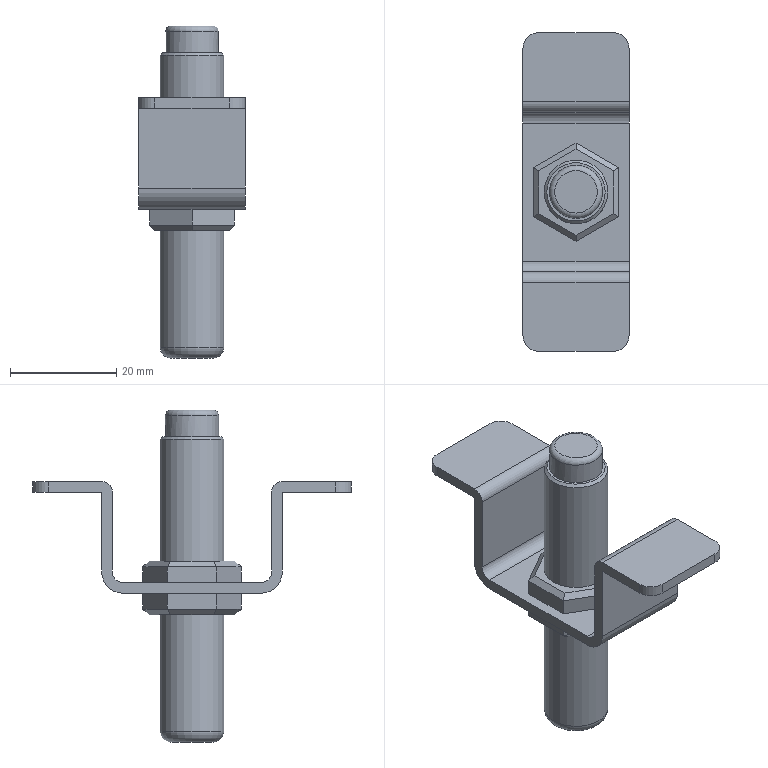Part | STEP file | Tube feed_id194_x_t | 1 solid | 59 faces | box 20 x 60 x 62.5 mm | volume 11212 mm3 | plane 43 | cylinder 13 | torus 2 | cone 1 | commonest cylinder face diameters 4 x4 6 x4 8 x2 12 x2 10 x1